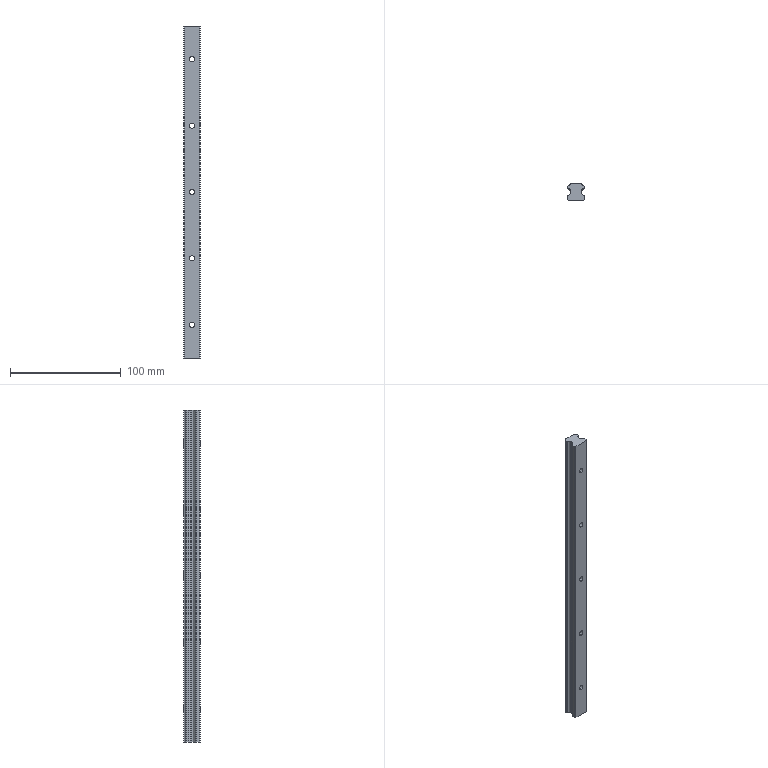Part | SolidWorks | features BaseBody 1 | 1 solid | 60 faces | box 15 x 15 x 300 mm | volume 55289 mm3 | cylinder 34 | plane 26 | commonest cylinder face diameters 4.5 x10 7.5 x10 0.8 x7 3.24 x4 2 x2 0.848 x1